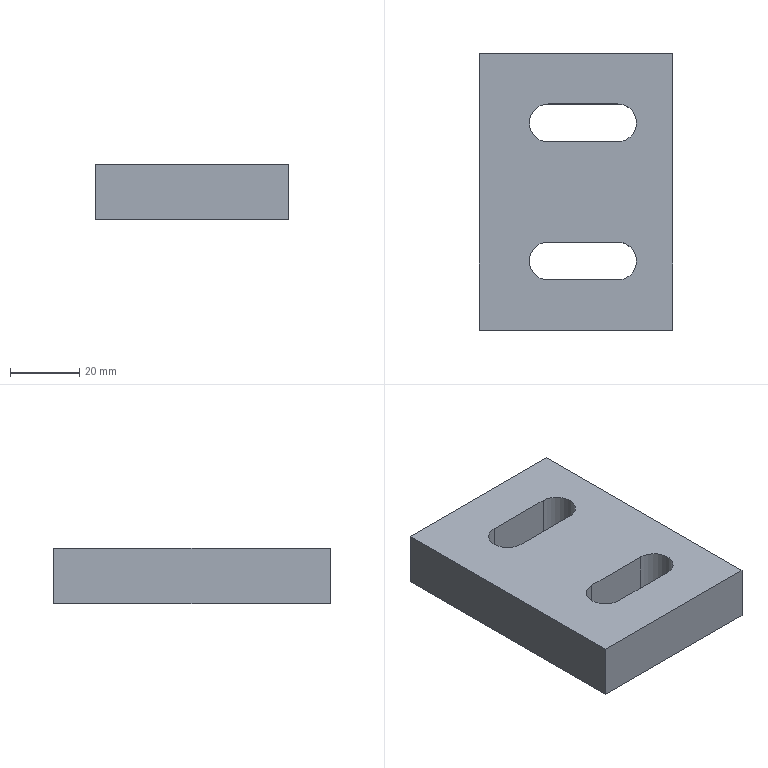Part | SolidWorks | features Extrusion 1, ICE 1 | 1 solid | 16 faces | box 56 x 80 x 16 mm | volume 61599 mm3 | plane 10 | cylinder 6 | commonest cylinder face diameters 11 x6
STEP:
#1=CARTESIAN_POINT('',(-13.5,20.,16.));
#2=VERTEX_POINT('',#1);
#3=CARTESIAN_POINT('',(-8.,25.5,16.));
#4=VERTEX_POINT('',#3);
#5=CARTESIAN_POINT('',(-8.,20.,16.));
#6=DIRECTION('',(0.,0.,-1.));
#7=DIRECTION('',(-1.,0.,0.));
#8=AXIS2_PLACEMENT_3D('',#5,#6,#7);
#9=CIRCLE('',#8,5.5);
#10=EDGE_CURVE('',#2,#4,#9,.T.);
#11=ORIENTED_EDGE('',*,*,#10,.F.);
#12=CARTESIAN_POINT('',(-13.5,20.,0.));
#13=VERTEX_POINT('',#12);
#14=CARTESIAN_POINT('',(-13.5,20.,16.));
#15=DIRECTION('',(0.,0.,-1.));
#16=VECTOR('',#15,1000.);
#17=LINE('',#14,#16);
#18=EDGE_CURVE('',#2,#13,#17,.T.);
#19=ORIENTED_EDGE('',*,*,#18,.T.);
#20=CARTESIAN_POINT('',(-8.,25.5,0.));
#21=VERTEX_POINT('',#20);
#22=CARTESIAN_POINT('',(-8.,20.,0.));
#23=DIRECTION('',(0.,0.,1.));
#24=DIRECTION('',(-1.,0.,0.));
#25=AXIS2_PLACEMENT_3D('',#22,#23,#24);
#26=CIRCLE('',#25,5.5);
#27=EDGE_CURVE('',#21,#13,#26,.T.);
#28=ORIENTED_EDGE('',*,*,#27,.F.);
#29=CARTESIAN_POINT('',(-8.,25.5,16.));
#30=DIRECTION('',(0.,0.,-1.));
#31=VECTOR('',#30,1000.);
#32=LINE('',#29,#31);
#33=EDGE_CURVE('',#4,#21,#32,.T.);
#34=ORIENTED_EDGE('',*,*,#33,.F.);
#35=EDGE_LOOP('',(#11,#19,#28,#34));
#36=FACE_OUTER_BOUND('',#35,.T.);
#37=CARTESIAN_POINT('',(-8.,20.,16.));
#38=DIRECTION('',(0.,0.,-1.));
#39=DIRECTION('',(-1.,0.,0.));
#40=AXIS2_PLACEMENT_3D('',#37,#38,#39);
#41=CYLINDRICAL_SURFACE('',#40,5.5);
#42=ADVANCED_FACE('',(#36),#41,.F.);
#43=CARTESIAN_POINT('',(-13.5,-20.,16.));
#44=VERTEX_POINT('',#43);
#45=CARTESIAN_POINT('',(-8.,-14.5,16.));
#46=VERTEX_POINT('',#45);
#47=CARTESIAN_POINT('',(-8.,-20.,16.));
#48=DIRECTION('',(0.,0.,-1.));
#49=DIRECTION('',(1.,0.,0.));
#50=AXIS2_PLACEMENT_3D('',#47,#48,#49);
#51=CIRCLE('',#50,5.5);
#52=EDGE_CURVE('',#44,#46,#51,.T.);
#53=ORIENTED_EDGE('',*,*,#52,.F.);
#54=CARTESIAN_POINT('',(-13.5,-20.,0.));
#55=VERTEX_POINT('',#54);
#56=CARTESIAN_POINT('',(-13.5,-20.,16.));
#57=DIRECTION('',(0.,0.,-1.));
#58=VECTOR('',#57,1000.);
#59=LINE('',#56,#58);
#60=EDGE_CURVE('',#44,#55,#59,.T.);
#61=ORIENTED_EDGE('',*,*,#60,.T.);
#62=CARTESIAN_POINT('',(-8.,-14.5,0.));
#63=VERTEX_POINT('',#62);
#64=CARTESIAN_POINT('',(-8.,-20.,0.));
#65=DIRECTION('',(0.,0.,1.));
#66=DIRECTION('',(-1.,0.,0.));
#67=AXIS2_PLACEMENT_3D('',#64,#65,#66);
#68=CIRCLE('',#67,5.5);
#69=EDGE_CURVE('',#63,#55,#68,.T.);
#70=ORIENTED_EDGE('',*,*,#69,.F.);
#71=CARTESIAN_POINT('',(-8.,-14.5,16.));
#72=DIRECTION('',(0.,0.,-1.));
#73=VECTOR('',#72,1000.);
#74=LINE('',#71,#73);
#75=EDGE_CURVE('',#46,#63,#74,.T.);
#76=ORIENTED_EDGE('',*,*,#75,.F.);
#77=EDGE_LOOP('',(#53,#61,#70,#76));
#78=FACE_OUTER_BOUND('',#77,.T.);
#79=CARTESIAN_POINT('',(-8.,-20.,16.));
#80=DIRECTION('',(0.,0.,-1.));
#81=DIRECTION('',(-1.,0.,0.));
#82=AXIS2_PLACEMENT_3D('',#79,#80,#81);
#83=CYLINDRICAL_SURFACE('',#82,5.5);
#84=ADVANCED_FACE('',(#78),#83,.F.);
#85=CARTESIAN_POINT('',(28.,-40.,0.));
#86=VERTEX_POINT('',#85);
#87=CARTESIAN_POINT('',(28.,40.,0.));
#88=VERTEX_POINT('',#87);
#89=CARTESIAN_POINT('',(28.,40.,0.));
#90=DIRECTION('',(0.,1.,0.));
#91=VECTOR('',#90,1000.);
#92=LINE('',#89,#91);
#93=EDGE_CURVE('',#86,#88,#92,.T.);
#94=ORIENTED_EDGE('',*,*,#93,.T.);
#95=CARTESIAN_POINT('',(28.,40.,16.));
#96=VERTEX_POINT('',#95);
#97=CARTESIAN_POINT('',(28.,40.,16.));
#98=DIRECTION('',(0.,0.,-1.));
#99=VECTOR('',#98,1000.);
#100=LINE('',#97,#99);
#101=EDGE_CURVE('',#96,#88,#100,.T.);
#102=ORIENTED_EDGE('',*,*,#101,.F.);
#103=CARTESIAN_POINT('',(28.,-40.,16.));
#104=VERTEX_POINT('',#103);
#105=CARTESIAN_POINT('',(28.,40.,16.));
#106=DIRECTION('',(0.,1.,0.));
#107=VECTOR('',#106,1000.);
#108=LINE('',#105,#107);
#109=EDGE_CURVE('',#104,#96,#108,.T.);
#110=ORIENTED_EDGE('',*,*,#109,.F.);
#111=CARTESIAN_POINT('',(28.,-40.,16.));
#112=DIRECTION('',(0.,0.,-1.));
#113=VECTOR('',#112,1000.);
#114=LINE('',#111,#113);
#115=EDGE_CURVE('',#104,#86,#114,.T.);
#116=ORIENTED_EDGE('',*,*,#115,.T.);
#117=EDGE_LOOP('',(#94,#102,#110,#116));
#118=FACE_OUTER_BOUND('',#117,.T.);
#119=CARTESIAN_POINT('',(28.,40.,16.));
#120=DIRECTION('',(-1.,0.,0.));
#121=DIRECTION('',(0.,-1.,0.));
#122=AXIS2_PLACEMENT_3D('',#119,#120,#121);
#123=PLANE('',#122);
#124=ADVANCED_FACE('',(#118),#123,.F.);
#125=CARTESIAN_POINT('',(-28.,40.,0.));
#126=VERTEX_POINT('',#125);
#127=CARTESIAN_POINT('',(-28.,40.,0.));
#128=DIRECTION('',(-1.,0.,0.));
#129=VECTOR('',#128,1000.);
#130=LINE('',#127,#129);
#131=EDGE_CURVE('',#88,#126,#130,.T.);
#132=ORIENTED_EDGE('',*,*,#131,.T.);
#133=CARTESIAN_POINT('',(-28.,40.,16.));
#134=VERTEX_POINT('',#133);
#135=CARTESIAN_POINT('',(-28.,40.,16.));
#136=DIRECTION('',(0.,0.,-1.));
#137=VECTOR('',#136,1000.);
#138=LINE('',#135,#137);
#139=EDGE_CURVE('',#134,#126,#138,.T.);
#140=ORIENTED_EDGE('',*,*,#139,.F.);
#141=CARTESIAN_POINT('',(-28.,40.,16.));
#142=DIRECTION('',(-1.,0.,0.));
#143=VECTOR('',#142,1000.);
#144=LINE('',#141,#143);
#145=EDGE_CURVE('',#96,#134,#144,.T.);
#146=ORIENTED_EDGE('',*,*,#145,.F.);
#147=ORIENTED_EDGE('',*,*,#101,.T.);
#148=EDGE_LOOP('',(#132,#140,#146,#147));
#149=FACE_OUTER_BOUND('',#148,.T.);
#150=CARTESIAN_POINT('',(-28.,40.,16.));
#151=DIRECTION('',(0.,-1.,0.));
#152=DIRECTION('',(0.,0.,-1.));
#153=AXIS2_PLACEMENT_3D('',#150,#151,#152);
#154=PLANE('',#153);
#155=ADVANCED_FACE('',(#149),#154,.F.);
#156=CARTESIAN_POINT('',(-28.,-40.,0.));
#157=VERTEX_POINT('',#156);
#158=CARTESIAN_POINT('',(-28.,40.,0.));
#159=DIRECTION('',(0.,-1.,0.));
#160=VECTOR('',#159,1000.);
#161=LINE('',#158,#160);
#162=EDGE_CURVE('',#126,#157,#161,.T.);
#163=ORIENTED_EDGE('',*,*,#162,.T.);
#164=CARTESIAN_POINT('',(-28.,-40.,16.));
#165=VERTEX_POINT('',#164);
#166=CARTESIAN_POINT('',(-28.,-40.,16.));
#167=DIRECTION('',(0.,0.,-1.));
#168=VECTOR('',#167,1000.);
#169=LINE('',#166,#168);
#170=EDGE_CURVE('',#165,#157,#169,.T.);
#171=ORIENTED_EDGE('',*,*,#170,.F.);
#172=CARTESIAN_POINT('',(-28.,40.,16.));
#173=DIRECTION('',(0.,-1.,0.));
#174=VECTOR('',#173,1000.);
#175=LINE('',#172,#174);
#176=EDGE_CURVE('',#134,#165,#175,.T.);
#177=ORIENTED_EDGE('',*,*,#176,.F.);
#178=ORIENTED_EDGE('',*,*,#139,.T.);
#179=EDGE_LOOP('',(#163,#171,#177,#178));
#180=FACE_OUTER_BOUND('',#179,.T.);
#181=CARTESIAN_POINT('',(-28.,40.,16.));
#182=DIRECTION('',(1.,0.,0.));
#183=DIRECTION('',(0.,1.,0.));
#184=AXIS2_PLACEMENT_3D('',#181,#182,#183);
#185=PLANE('',#184);
#186=ADVANCED_FACE('',(#180),#185,.F.);
#187=CARTESIAN_POINT('',(-28.,-40.,0.));
#188=DIRECTION('',(1.,0.,0.));
#189=VECTOR('',#188,1000.);
#190=LINE('',#187,#189);
#191=EDGE_CURVE('',#157,#86,#190,.T.);
#192=ORIENTED_EDGE('',*,*,#191,.T.);
#193=ORIENTED_EDGE('',*,*,#115,.F.);
#194=CARTESIAN_POINT('',(-28.,-40.,16.));
#195=DIRECTION('',(1.,0.,0.));
#196=VECTOR('',#195,1000.);
#197=LINE('',#194,#196);
#198=EDGE_CURVE('',#165,#104,#197,.T.);
#199=ORIENTED_EDGE('',*,*,#198,.F.);
#200=ORIENTED_EDGE('',*,*,#170,.T.);
#201=EDGE_LOOP('',(#192,#193,#199,#200));
#202=FACE_OUTER_BOUND('',#201,.T.);
#203=CARTESIAN_POINT('',(-28.,-40.,16.));
#204=DIRECTION('',(0.,1.,0.));
#205=DIRECTION('',(0.,0.,1.));
#206=AXIS2_PLACEMENT_3D('',#203,#204,#205);
#207=PLANE('',#206);
#208=ADVANCED_FACE('',(#202),#207,.F.);
#209=CARTESIAN_POINT('',(12.,25.5,16.));
#210=VERTEX_POINT('',#209);
#211=CARTESIAN_POINT('',(12.,14.5,16.));
#212=VERTEX_POINT('',#211);
#213=CARTESIAN_POINT('',(12.,20.,16.));
#214=DIRECTION('',(0.,0.,-1.));
#215=DIRECTION('',(-1.,0.,0.));
#216=AXIS2_PLACEMENT_3D('',#213,#214,#215);
#217=CIRCLE('',#216,5.5);
#218=EDGE_CURVE('',#210,#212,#217,.T.);
#219=ORIENTED_EDGE('',*,*,#218,.T.);
#220=CARTESIAN_POINT('',(-8.,14.5,16.));
#221=VERTEX_POINT('',#220);
#222=CARTESIAN_POINT('',(12.,14.5,16.));
#223=DIRECTION('',(-1.,0.,0.));
#224=VECTOR('',#223,1000.);
#225=LINE('',#222,#224);
#226=EDGE_CURVE('',#212,#221,#225,.T.);
#227=ORIENTED_EDGE('',*,*,#226,.T.);
#228=CARTESIAN_POINT('',(-8.,20.,16.));
#229=DIRECTION('',(0.,0.,-1.));
#230=DIRECTION('',(-1.,0.,0.));
#231=AXIS2_PLACEMENT_3D('',#228,#229,#230);
#232=CIRCLE('',#231,5.5);
#233=EDGE_CURVE('',#221,#2,#232,.T.);
#234=ORIENTED_EDGE('',*,*,#233,.T.);
#235=ORIENTED_EDGE('',*,*,#10,.T.);
#236=CARTESIAN_POINT('',(12.,25.5,16.));
#237=DIRECTION('',(1.,0.,0.));
#238=VECTOR('',#237,1000.);
#239=LINE('',#236,#238);
#240=EDGE_CURVE('',#4,#210,#239,.T.);
#241=ORIENTED_EDGE('',*,*,#240,.T.);
#242=EDGE_LOOP('',(#219,#227,#234,#235,#241));
#243=FACE_BOUND('',#242,.T.);
#244=CARTESIAN_POINT('',(12.,-14.5,16.));
#245=VERTEX_POINT('',#244);
#246=CARTESIAN_POINT('',(12.,-25.5,16.));
#247=VERTEX_POINT('',#246);
#248=CARTESIAN_POINT('',(12.,-20.,16.));
#249=DIRECTION('',(0.,0.,-1.));
#250=DIRECTION('',(1.,0.,0.));
#251=AXIS2_PLACEMENT_3D('',#248,#249,#250);
#252=CIRCLE('',#251,5.5);
#253=EDGE_CURVE('',#245,#247,#252,.T.);
#254=ORIENTED_EDGE('',*,*,#253,.T.);
#255=CARTESIAN_POINT('',(-8.,-25.5,16.));
#256=VERTEX_POINT('',#255);
#257=CARTESIAN_POINT('',(12.,-25.5,16.));
#258=DIRECTION('',(-1.,0.,0.));
#259=VECTOR('',#258,1000.);
#260=LINE('',#257,#259);
#261=EDGE_CURVE('',#247,#256,#260,.T.);
#262=ORIENTED_EDGE('',*,*,#261,.T.);
#263=CARTESIAN_POINT('',(-8.,-20.,16.));
#264=DIRECTION('',(0.,0.,-1.));
#265=DIRECTION('',(1.,0.,0.));
#266=AXIS2_PLACEMENT_3D('',#263,#264,#265);
#267=CIRCLE('',#266,5.5);
#268=EDGE_CURVE('',#256,#44,#267,.T.);
#269=ORIENTED_EDGE('',*,*,#268,.T.);
#270=ORIENTED_EDGE('',*,*,#52,.T.);
#271=CARTESIAN_POINT('',(12.,-14.5,16.));
#272=DIRECTION('',(1.,0.,0.));
#273=VECTOR('',#272,1000.);
#274=LINE('',#271,#273);
#275=EDGE_CURVE('',#46,#245,#274,.T.);
#276=ORIENTED_EDGE('',*,*,#275,.T.);
#277=EDGE_LOOP('',(#254,#262,#269,#270,#276));
#278=FACE_BOUND('',#277,.T.);
#279=ORIENTED_EDGE('',*,*,#109,.T.);
#280=ORIENTED_EDGE('',*,*,#145,.T.);
#281=ORIENTED_EDGE('',*,*,#176,.T.);
#282=ORIENTED_EDGE('',*,*,#198,.T.);
#283=EDGE_LOOP('',(#279,#280,#281,#282));
#284=FACE_OUTER_BOUND('',#283,.T.);
#285=CARTESIAN_POINT('',(0.,0.,16.));
#286=DIRECTION('',(0.,0.,1.));
#287=DIRECTION('',(1.,0.,0.));
#288=AXIS2_PLACEMENT_3D('',#285,#286,#287);
#289=PLANE('',#288);
#290=ADVANCED_FACE('',(#243,#278,#284),#289,.T.);
#291=CARTESIAN_POINT('',(-8.,14.5,0.));
#292=VERTEX_POINT('',#291);
#293=CARTESIAN_POINT('',(12.,14.5,0.));
#294=VERTEX_POINT('',#293);
#295=CARTESIAN_POINT('',(0.,14.5,0.));
#296=DIRECTION('',(1.,0.,0.));
#297=VECTOR('',#296,1000.);
#298=LINE('',#295,#297);
#299=EDGE_CURVE('',#292,#294,#298,.T.);
#300=ORIENTED_EDGE('',*,*,#299,.T.);
#301=CARTESIAN_POINT('',(12.,25.5,0.));
#302=VERTEX_POINT('',#301);
#303=CARTESIAN_POINT('',(12.,20.,0.));
#304=DIRECTION('',(0.,0.,1.));
#305=DIRECTION('',(-1.,0.,0.));
#306=AXIS2_PLACEMENT_3D('',#303,#304,#305);
#307=CIRCLE('',#306,5.5);
#308=EDGE_CURVE('',#294,#302,#307,.T.);
#309=ORIENTED_EDGE('',*,*,#308,.T.);
#310=CARTESIAN_POINT('',(0.,25.5,0.));
#311=DIRECTION('',(-1.,0.,0.));
#312=VECTOR('',#311,1000.);
#313=LINE('',#310,#312);
#314=EDGE_CURVE('',#302,#21,#313,.T.);
#315=ORIENTED_EDGE('',*,*,#314,.T.);
#316=ORIENTED_EDGE('',*,*,#27,.T.);
#317=CARTESIAN_POINT('',(-8.,20.,0.));
#318=DIRECTION('',(0.,0.,1.));
#319=DIRECTION('',(-1.,0.,0.));
#320=AXIS2_PLACEMENT_3D('',#317,#318,#319);
#321=CIRCLE('',#320,5.5);
#322=EDGE_CURVE('',#13,#292,#321,.T.);
#323=ORIENTED_EDGE('',*,*,#322,.T.);
#324=EDGE_LOOP('',(#300,#309,#315,#316,#323));
#325=FACE_BOUND('',#324,.T.);
#326=CARTESIAN_POINT('',(-8.,-25.5,0.));
#327=VERTEX_POINT('',#326);
#328=CARTESIAN_POINT('',(12.,-25.5,0.));
#329=VERTEX_POINT('',#328);
#330=CARTESIAN_POINT('',(0.,-25.5,0.));
#331=DIRECTION('',(1.,0.,0.));
#332=VECTOR('',#331,1000.);
#333=LINE('',#330,#332);
#334=EDGE_CURVE('',#327,#329,#333,.T.);
#335=ORIENTED_EDGE('',*,*,#334,.T.);
#336=CARTESIAN_POINT('',(12.,-14.5,0.));
#337=VERTEX_POINT('',#336);
#338=CARTESIAN_POINT('',(12.,-20.,0.));
#339=DIRECTION('',(0.,0.,1.));
#340=DIRECTION('',(-1.,0.,0.));
#341=AXIS2_PLACEMENT_3D('',#338,#339,#340);
#342=CIRCLE('',#341,5.5);
#343=EDGE_CURVE('',#329,#337,#342,.T.);
#344=ORIENTED_EDGE('',*,*,#343,.T.);
#345=CARTESIAN_POINT('',(0.,-14.5,0.));
#346=DIRECTION('',(-1.,0.,0.));
#347=VECTOR('',#346,1000.);
#348=LINE('',#345,#347);
#349=EDGE_CURVE('',#337,#63,#348,.T.);
#350=ORIENTED_EDGE('',*,*,#349,.T.);
#351=ORIENTED_EDGE('',*,*,#69,.T.);
#352=CARTESIAN_POINT('',(-8.,-20.,0.));
#353=DIRECTION('',(0.,0.,1.));
#354=DIRECTION('',(-1.,0.,0.));
#355=AXIS2_PLACEMENT_3D('',#352,#353,#354);
#356=CIRCLE('',#355,5.5);
#357=EDGE_CURVE('',#55,#327,#356,.T.);
#358=ORIENTED_EDGE('',*,*,#357,.T.);
#359=EDGE_LOOP('',(#335,#344,#350,#351,#358));
#360=FACE_BOUND('',#359,.T.);
#361=ORIENTED_EDGE('',*,*,#93,.F.);
#362=ORIENTED_EDGE('',*,*,#191,.F.);
#363=ORIENTED_EDGE('',*,*,#162,.F.);
#364=ORIENTED_EDGE('',*,*,#131,.F.);
#365=EDGE_LOOP('',(#361,#362,#363,#364));
#366=FACE_OUTER_BOUND('',#365,.T.);
#367=CARTESIAN_POINT('',(0.,0.,0.));
#368=DIRECTION('',(0.,0.,1.));
#369=DIRECTION('',(1.,0.,0.));
#370=AXIS2_PLACEMENT_3D('',#367,#368,#369);
#371=PLANE('',#370);
#372=ADVANCED_FACE('',(#325,#360,#366),#371,.F.);
#373=CARTESIAN_POINT('',(12.,-25.5,16.));
#374=DIRECTION('',(0.,0.,-1.));
#375=VECTOR('',#374,1000.);
#376=LINE('',#373,#375);
#377=EDGE_CURVE('',#247,#329,#376,.T.);
#378=ORIENTED_EDGE('',*,*,#377,.F.);
#379=ORIENTED_EDGE('',*,*,#253,.F.);
#380=CARTESIAN_POINT('',(12.,-14.5,16.));
#381=DIRECTION('',(0.,0.,-1.));
#382=VECTOR('',#381,1000.);
#383=LINE('',#380,#382);
#384=EDGE_CURVE('',#245,#337,#383,.T.);
#385=ORIENTED_EDGE('',*,*,#384,.T.);
#386=ORIENTED_EDGE('',*,*,#343,.F.);
#387=EDGE_LOOP('',(#378,#379,#385,#386));
#388=FACE_OUTER_BOUND('',#387,.T.);
#389=CARTESIAN_POINT('',(12.,-20.,16.));
#390=DIRECTION('',(0.,0.,-1.));
#391=DIRECTION('',(-1.,0.,0.));
#392=AXIS2_PLACEMENT_3D('',#389,#390,#391);
#393=CYLINDRICAL_SURFACE('',#392,5.5);
#394=ADVANCED_FACE('',(#388),#393,.F.);
#395=ORIENTED_EDGE('',*,*,#384,.F.);
#396=ORIENTED_EDGE('',*,*,#275,.F.);
#397=ORIENTED_EDGE('',*,*,#75,.T.);
#398=ORIENTED_EDGE('',*,*,#349,.F.);
#399=EDGE_LOOP('',(#395,#396,#397,#398));
#400=FACE_OUTER_BOUND('',#399,.T.);
#401=CARTESIAN_POINT('',(12.,-14.5,16.));
#402=DIRECTION('',(0.,1.,0.));
#403=DIRECTION('',(-1.,0.,0.));
#404=AXIS2_PLACEMENT_3D('',#401,#402,#403);
#405=PLANE('',#404);
#406=ADVANCED_FACE('',(#400),#405,.F.);
#407=ORIENTED_EDGE('',*,*,#60,.F.);
#408=ORIENTED_EDGE('',*,*,#268,.F.);
#409=CARTESIAN_POINT('',(-8.,-25.5,16.));
#410=DIRECTION('',(0.,0.,-1.));
#411=VECTOR('',#410,1000.);
#412=LINE('',#409,#411);
#413=EDGE_CURVE('',#256,#327,#412,.T.);
#414=ORIENTED_EDGE('',*,*,#413,.T.);
#415=ORIENTED_EDGE('',*,*,#357,.F.);
#416=EDGE_LOOP('',(#407,#408,#414,#415));
#417=FACE_OUTER_BOUND('',#416,.T.);
#418=CARTESIAN_POINT('',(-8.,-20.,16.));
#419=DIRECTION('',(0.,0.,-1.));
#420=DIRECTION('',(-1.,0.,0.));
#421=AXIS2_PLACEMENT_3D('',#418,#419,#420);
#422=CYLINDRICAL_SURFACE('',#421,5.5);
#423=ADVANCED_FACE('',(#417),#422,.F.);
#424=ORIENTED_EDGE('',*,*,#413,.F.);
#425=ORIENTED_EDGE('',*,*,#261,.F.);
#426=ORIENTED_EDGE('',*,*,#377,.T.);
#427=ORIENTED_EDGE('',*,*,#334,.F.);
#428=EDGE_LOOP('',(#424,#425,#426,#427));
#429=FACE_OUTER_BOUND('',#428,.T.);
#430=CARTESIAN_POINT('',(12.,-25.5,16.));
#431=DIRECTION('',(0.,-1.,0.));
#432=DIRECTION('',(1.,0.,0.));
#433=AXIS2_PLACEMENT_3D('',#430,#431,#432);
#434=PLANE('',#433);
#435=ADVANCED_FACE('',(#429),#434,.F.);
#436=CARTESIAN_POINT('',(12.,14.5,16.));
#437=DIRECTION('',(0.,0.,-1.));
#438=VECTOR('',#437,1000.);
#439=LINE('',#436,#438);
#440=EDGE_CURVE('',#212,#294,#439,.T.);
#441=ORIENTED_EDGE('',*,*,#440,.F.);
#442=ORIENTED_EDGE('',*,*,#218,.F.);
#443=CARTESIAN_POINT('',(12.,25.5,16.));
#444=DIRECTION('',(0.,0.,-1.));
#445=VECTOR('',#444,1000.);
#446=LINE('',#443,#445);
#447=EDGE_CURVE('',#210,#302,#446,.T.);
#448=ORIENTED_EDGE('',*,*,#447,.T.);
#449=ORIENTED_EDGE('',*,*,#308,.F.);
#450=EDGE_LOOP('',(#441,#442,#448,#449));
#451=FACE_OUTER_BOUND('',#450,.T.);
#452=CARTESIAN_POINT('',(12.,20.,16.));
#453=DIRECTION('',(0.,0.,-1.));
#454=DIRECTION('',(-1.,0.,0.));
#455=AXIS2_PLACEMENT_3D('',#452,#453,#454);
#456=CYLINDRICAL_SURFACE('',#455,5.5);
#457=ADVANCED_FACE('',(#451),#456,.F.);
#458=ORIENTED_EDGE('',*,*,#447,.F.);
#459=ORIENTED_EDGE('',*,*,#240,.F.);
#460=ORIENTED_EDGE('',*,*,#33,.T.);
#461=ORIENTED_EDGE('',*,*,#314,.F.);
#462=EDGE_LOOP('',(#458,#459,#460,#461));
#463=FACE_OUTER_BOUND('',#462,.T.);
#464=CARTESIAN_POINT('',(12.,25.5,16.));
#465=DIRECTION('',(0.,1.,0.));
#466=DIRECTION('',(-1.,0.,0.));
#467=AXIS2_PLACEMENT_3D('',#464,#465,#466);
#468=PLANE('',#467);
#469=ADVANCED_FACE('',(#463),#468,.F.);
#470=ORIENTED_EDGE('',*,*,#18,.F.);
#471=ORIENTED_EDGE('',*,*,#233,.F.);
#472=CARTESIAN_POINT('',(-8.,14.5,16.));
#473=DIRECTION('',(0.,0.,-1.));
#474=VECTOR('',#473,1000.);
#475=LINE('',#472,#474);
#476=EDGE_CURVE('',#221,#292,#475,.T.);
#477=ORIENTED_EDGE('',*,*,#476,.T.);
#478=ORIENTED_EDGE('',*,*,#322,.F.);
#479=EDGE_LOOP('',(#470,#471,#477,#478));
#480=FACE_OUTER_BOUND('',#479,.T.);
#481=CARTESIAN_POINT('',(-8.,20.,16.));
#482=DIRECTION('',(0.,0.,-1.));
#483=DIRECTION('',(-1.,0.,0.));
#484=AXIS2_PLACEMENT_3D('',#481,#482,#483);
#485=CYLINDRICAL_SURFACE('',#484,5.5);
#486=ADVANCED_FACE('',(#480),#485,.F.);
#487=ORIENTED_EDGE('',*,*,#476,.F.);
#488=ORIENTED_EDGE('',*,*,#226,.F.);
#489=ORIENTED_EDGE('',*,*,#440,.T.);
#490=ORIENTED_EDGE('',*,*,#299,.F.);
#491=EDGE_LOOP('',(#487,#488,#489,#490));
#492=FACE_OUTER_BOUND('',#491,.T.);
#493=CARTESIAN_POINT('',(12.,14.5,16.));
#494=DIRECTION('',(0.,-1.,0.));
#495=DIRECTION('',(1.,0.,0.));
#496=AXIS2_PLACEMENT_3D('',#493,#494,#495);
#497=PLANE('',#496);
#498=ADVANCED_FACE('',(#492),#497,.F.);
#499=CLOSED_SHELL('',(#42,#84,#124,#155,#186,#208,#290,#372,#394,#406,#423,#435,#457,#469,#486,#498));
#500=MANIFOLD_SOLID_BREP('',#499);
#501=CARTESIAN_POINT('',(0.,0.,0.));
#502=DIRECTION('',(0.,0.,1.));
#503=DIRECTION('',(1.,0.,0.));
#504=AXIS2_PLACEMENT_3D('',#501,#502,#503);
#505=(LENGTH_UNIT()NAMED_UNIT(*)SI_UNIT(.MILLI.,.METRE.));
#506=UNCERTAINTY_MEASURE_WITH_UNIT(LENGTH_MEASURE(0.00001),#505,'','');
#507=(NAMED_UNIT(*)PLANE_ANGLE_UNIT()SI_UNIT($,.RADIAN.));
#508=(NAMED_UNIT(*)SI_UNIT($,.STERADIAN.)SOLID_ANGLE_UNIT());
#509=(GEOMETRIC_REPRESENTATION_CONTEXT(3)GLOBAL_UNCERTAINTY_ASSIGNED_CONTEXT((#506))GLOBAL_UNIT_ASSIGNED_CONTEXT((#505,#507,#508))REPRESENTATION_CONTEXT('',''));
#510=ADVANCED_BREP_SHAPE_REPRESENTATION('',(#500,#504),#509);